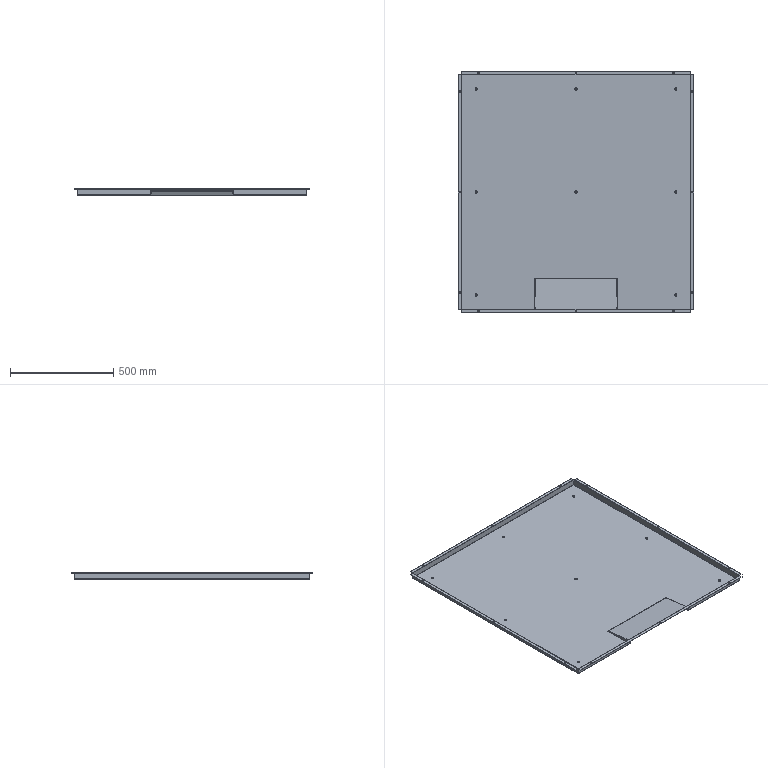Part | 2 solids | 170 faces | box 1140 x 1170 x 30.147 mm | volume 1453893 mm3 | plane 90 | cylinder 68 | spline 12 | commonest cylinder face diameters 7 x30 11 x16 0.4 x9 2.4 x9 2 x2 4 x2